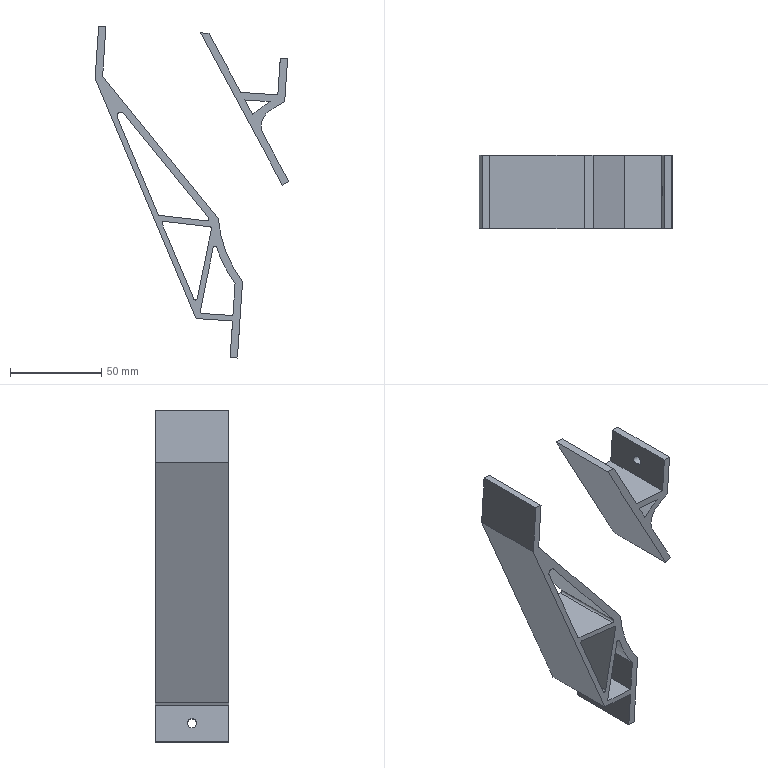Part | STEP file | Chuck limit ring | 2 solids | 52 faces | box 105.924 x 40 x 181.464 mm | volume 85930 mm3 | plane 33 | cylinder 19 | commonest cylinder face diameters 2 x8 5.1 x4 4 x2 130 x2 138 x2 20 x1